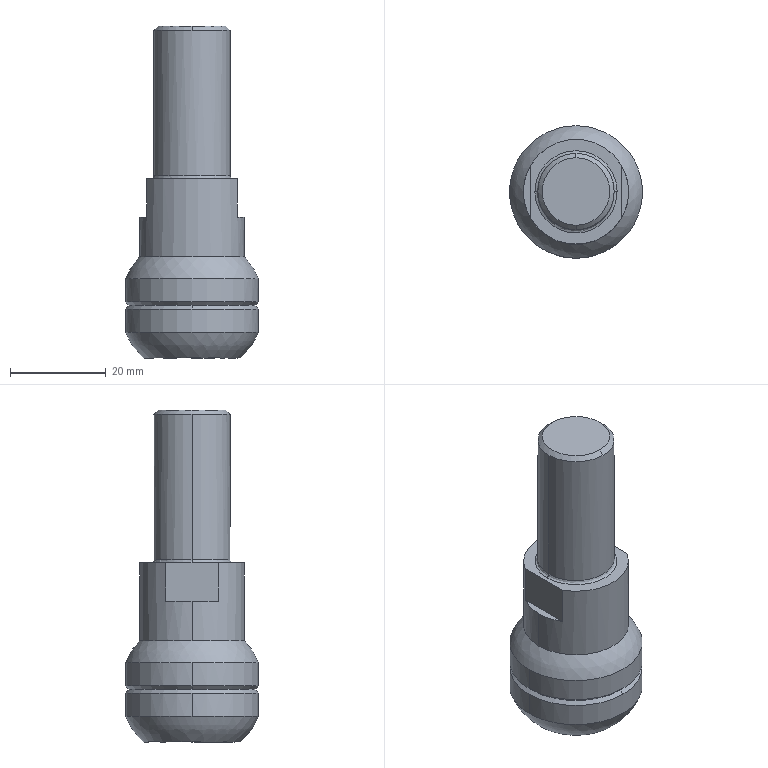Part | SolidWorks | features BaseBody 1 | 1 solid | 25 faces | box 27.8 x 27.8 x 69.5 mm | volume 24116 mm3 | cylinder 8 | plane 7 | cone 6 | spline 4 | commonest cylinder face diameters 27.8 x4 16 x2 22 x2
STEP:
#1=CARTESIAN_POINT('',(8.,0.,0.6));
#2=VERTEX_POINT('',#1);
#3=CARTESIAN_POINT('',(-8.,0.,0.6));
#4=VERTEX_POINT('',#3);
#5=CARTESIAN_POINT('',(0.,0.,0.6));
#6=DIRECTION('',(0.,0.,1.));
#7=DIRECTION('',(1.,0.,0.));
#8=AXIS2_PLACEMENT_3D('',#5,#6,#7);
#9=CIRCLE('',#8,8.);
#10=EDGE_CURVE('',#2,#4,#9,.T.);
#11=ORIENTED_EDGE('',*,*,#10,.F.);
#12=CARTESIAN_POINT('',(8.6,0.,0.));
#13=VERTEX_POINT('',#12);
#14=CARTESIAN_POINT('',(8.6,0.,0.6));
#15=DIRECTION('',(0.,-1.,0.));
#16=DIRECTION('',(1.,0.,0.));
#17=AXIS2_PLACEMENT_3D('',#14,#15,#16);
#18=CIRCLE('',#17,0.6);
#19=EDGE_CURVE('',#2,#13,#18,.T.);
#20=ORIENTED_EDGE('',*,*,#19,.T.);
#21=CARTESIAN_POINT('',(-8.6,0.,0.));
#22=VERTEX_POINT('',#21);
#23=CARTESIAN_POINT('',(-8.6,0.,0.));
#24=CARTESIAN_POINT('',(-8.6,0.2629,0.));
#25=CARTESIAN_POINT('',(-8.582,0.6557,0.));
#26=CARTESIAN_POINT('',(-8.53,1.111,0.));
#27=CARTESIAN_POINT('',(-8.496,1.338,0.));
#28=CARTESIAN_POINT('',(-8.479,1.435,0.));
#29=CARTESIAN_POINT('',(-8.468,1.5,0.));
#30=CARTESIAN_POINT('',(-8.463,1.531,0.));
#31=CARTESIAN_POINT('',(-8.406,1.839,0.));
#32=CARTESIAN_POINT('',(-8.31,2.245,0.));
#33=CARTESIAN_POINT('',(-8.164,2.709,0.));
#34=CARTESIAN_POINT('',(-8.083,2.938,0.));
#35=CARTESIAN_POINT('',(-8.046,3.036,0.));
#36=CARTESIAN_POINT('',(-8.022,3.101,0.));
#37=CARTESIAN_POINT('',(-8.01,3.132,0.));
#38=CARTESIAN_POINT('',(-7.889,3.436,0.));
#39=CARTESIAN_POINT('',(-7.709,3.831,0.));
#40=CARTESIAN_POINT('',(-7.465,4.275,0.));
#41=CARTESIAN_POINT('',(-7.353,4.461,0.));
#42=CARTESIAN_POINT('',(-7.277,4.584,0.));
#43=CARTESIAN_POINT('',(-7.239,4.644,0.));
#44=CARTESIAN_POINT('',(-6.873,5.203,0.));
#45=CARTESIAN_POINT('',(-6.501,5.661,0.));
#46=CARTESIAN_POINT('',(-5.871,6.291,0.));
#47=CARTESIAN_POINT('',(-5.542,6.588,0.));
#48=CARTESIAN_POINT('',(-5.132,6.904,0.));
#49=CARTESIAN_POINT('',(-4.951,7.032,0.));
#50=CARTESIAN_POINT('',(-4.83,7.116,0.));
#51=CARTESIAN_POINT('',(-4.767,7.158,0.));
#52=CARTESIAN_POINT('',(-4.463,7.357,0.));
#53=CARTESIAN_POINT('',(-4.087,7.576,0.));
#54=CARTESIAN_POINT('',(-3.632,7.798,0.));
#55=CARTESIAN_POINT('',(-3.4,7.9,0.));
#56=CARTESIAN_POINT('',(-3.3,7.942,0.));
#57=CARTESIAN_POINT('',(-3.233,7.969,0.));
#58=CARTESIAN_POINT('',(-3.198,7.983,0.));
#59=CARTESIAN_POINT('',(-2.906,8.099,0.));
#60=CARTESIAN_POINT('',(-2.511,8.233,0.));
#61=CARTESIAN_POINT('',(-2.041,8.356,0.));
#62=CARTESIAN_POINT('',(-1.804,8.409,0.));
#63=CARTESIAN_POINT('',(-1.702,8.43,0.));
#64=CARTESIAN_POINT('',(-1.633,8.444,0.));
#65=CARTESIAN_POINT('',(-1.597,8.45,0.));
#66=CARTESIAN_POINT('',(-1.047,8.552,0.));
#67=CARTESIAN_POINT('',(-0.5264,8.6,0.));
#68=CARTESIAN_POINT('',(0.2632,8.6,0.));
#69=CARTESIAN_POINT('',(0.6562,8.582,0.));
#70=CARTESIAN_POINT('',(1.112,8.53,0.));
#71=CARTESIAN_POINT('',(1.338,8.496,0.));
#72=CARTESIAN_POINT('',(1.436,8.479,0.));
#73=CARTESIAN_POINT('',(1.5,8.468,0.));
#74=CARTESIAN_POINT('',(1.531,8.463,0.));
#75=CARTESIAN_POINT('',(1.839,8.406,0.));
#76=CARTESIAN_POINT('',(2.245,8.31,0.));
#77=CARTESIAN_POINT('',(2.709,8.164,0.));
#78=CARTESIAN_POINT('',(2.938,8.083,0.));
#79=CARTESIAN_POINT('',(3.036,8.046,0.));
#80=CARTESIAN_POINT('',(3.101,8.022,0.));
#81=CARTESIAN_POINT('',(3.132,8.01,0.));
#82=CARTESIAN_POINT('',(3.436,7.889,0.));
#83=CARTESIAN_POINT('',(3.831,7.709,0.));
#84=CARTESIAN_POINT('',(4.275,7.465,0.));
#85=CARTESIAN_POINT('',(4.461,7.353,0.));
#86=CARTESIAN_POINT('',(4.584,7.277,0.));
#87=CARTESIAN_POINT('',(4.644,7.239,0.));
#88=CARTESIAN_POINT('',(5.203,6.873,0.));
#89=CARTESIAN_POINT('',(5.661,6.501,0.));
#90=CARTESIAN_POINT('',(6.291,5.871,0.));
#91=CARTESIAN_POINT('',(6.588,5.542,0.));
#92=CARTESIAN_POINT('',(6.904,5.132,0.));
#93=CARTESIAN_POINT('',(7.032,4.951,0.));
#94=CARTESIAN_POINT('',(7.116,4.83,0.));
#95=CARTESIAN_POINT('',(7.158,4.767,0.));
#96=CARTESIAN_POINT('',(7.357,4.463,0.));
#97=CARTESIAN_POINT('',(7.576,4.087,0.));
#98=CARTESIAN_POINT('',(7.798,3.632,0.));
#99=CARTESIAN_POINT('',(7.9,3.4,0.));
#100=CARTESIAN_POINT('',(7.942,3.3,0.));
#101=CARTESIAN_POINT('',(7.969,3.233,0.));
#102=CARTESIAN_POINT('',(7.983,3.198,0.));
#103=CARTESIAN_POINT('',(8.099,2.906,0.));
#104=CARTESIAN_POINT('',(8.233,2.511,0.));
#105=CARTESIAN_POINT('',(8.356,2.041,0.));
#106=CARTESIAN_POINT('',(8.409,1.804,0.));
#107=CARTESIAN_POINT('',(8.43,1.702,0.));
#108=CARTESIAN_POINT('',(8.444,1.633,0.));
#109=CARTESIAN_POINT('',(8.45,1.597,0.));
#110=CARTESIAN_POINT('',(8.552,1.047,0.));
#111=CARTESIAN_POINT('',(8.6,0.5264,0.));
#112=CARTESIAN_POINT('',(8.6,0.,0.));
#113=B_SPLINE_CURVE_WITH_KNOTS('',3,(#23,#24,#25,#26,#27,#28,#29,#30,#31,#32,#33,#34,#35,#36,#37,#38,#39,#40,#41,#42,#43,#44,#45,#46,#47,#48,#49,#50,#51,#52,#53,#54,#55,#56,#57,#58,#59,#60,#61,#62,#63,#64,#65,#66,#67,#68,#69,#70,#71,#72,#73,#74,#75,#76,#77,#78,#79,#80,#81,#82,#83,#84,#85,#86,#87,#88,#89,#90,#91,#92,#93,#94,#95,#96,#97,#98,#99,#100,#101,#102,#103,#104,#105,#106,#107,#108,#109,#110,#111,#112),.UNSPECIFIED.,.F.,.F.,(4,1,1,1,2,2,1,1,1,2,2,1,1,2,2,2,1,1,2,2,1,1,1,2,2,1,1,1,2,2,2,1,1,1,2,2,1,1,1,2,2,1,1,2,2,2,1,1,2,2,1,1,1,2,2,1,1,1,2,2,4),(0.,0.01563,0.02344,0.02734,0.0293,0.03125,0.04688,0.05469,0.05859,0.06055,0.0625,0.07813,0.08594,0.08984,0.09375,0.125,0.1406,0.1484,0.1523,0.1563,0.1719,0.1797,0.1836,0.1855,0.1875,0.2031,0.2109,0.2148,0.2168,0.2188,0.25,0.2656,0.2734,0.2773,0.2793,0.2813,0.2969,0.3047,0.3086,0.3105,0.3125,0.3281,0.3359,0.3398,0.3438,0.375,0.3906,0.3984,0.4023,0.4063,0.4219,0.4297,0.4336,0.4355,0.4375,0.4531,0.4609,0.4648,0.4668,0.4688,0.5),.UNSPECIFIED.);
#114=EDGE_CURVE('',#22,#13,#113,.T.);
#115=ORIENTED_EDGE('',*,*,#114,.F.);
#116=CARTESIAN_POINT('',(-8.6,0.,0.6));
#117=DIRECTION('',(0.,1.,0.));
#118=DIRECTION('',(-1.,0.,0.));
#119=AXIS2_PLACEMENT_3D('',#116,#117,#118);
#120=CIRCLE('',#119,0.6);
#121=EDGE_CURVE('',#4,#22,#120,.T.);
#122=ORIENTED_EDGE('',*,*,#121,.F.);
#123=EDGE_LOOP('',(#11,#20,#115,#122));
#124=FACE_OUTER_BOUND('',#123,.T.);
#125=CARTESIAN_POINT('',(-8.,0.,0.6));
#126=CARTESIAN_POINT('',(-8.,16.,0.6));
#127=CARTESIAN_POINT('',(8.,16.,0.6));
#128=CARTESIAN_POINT('',(8.,0.,0.6));
#129=CARTESIAN_POINT('',(-8.,0.,0.2485));
#130=CARTESIAN_POINT('',(-8.,16.,0.2485));
#131=CARTESIAN_POINT('',(8.,16.,0.2485));
#132=CARTESIAN_POINT('',(8.,0.,0.2485));
#133=CARTESIAN_POINT('',(-8.249,0.,0.));
#134=CARTESIAN_POINT('',(-8.249,16.497,0.));
#135=CARTESIAN_POINT('',(8.249,16.497,0.));
#136=CARTESIAN_POINT('',(8.249,0.,0.));
#137=CARTESIAN_POINT('',(-8.6,0.,0.));
#138=CARTESIAN_POINT('',(-8.6,17.2,0.));
#139=CARTESIAN_POINT('',(8.6,17.2,0.));
#140=CARTESIAN_POINT('',(8.6,0.,0.));
#141=(BOUNDED_SURFACE()B_SPLINE_SURFACE(3,3,((#125,#126,#127,#128),(#129,#130,#131,#132),(#133,#134,#135,#136),(#137,#138,#139,#140)),.UNSPECIFIED.,.F.,.F.,.F.)B_SPLINE_SURFACE_WITH_KNOTS((4,4),(4,4),(0.,1.),(0.,1.),.UNSPECIFIED.)GEOMETRIC_REPRESENTATION_ITEM()RATIONAL_B_SPLINE_SURFACE(((1.,0.3333,0.3333,1.),(0.8047,0.2682,0.2682,0.8047),(0.8047,0.2682,0.2682,0.8047),(1.,0.3333,0.3333,1.)))REPRESENTATION_ITEM('')SURFACE());
#142=ADVANCED_FACE('',(#124),#141,.F.);
#143=ORIENTED_EDGE('',*,*,#10,.T.);
#144=CARTESIAN_POINT('',(-8.,0.,31.08));
#145=VERTEX_POINT('',#144);
#146=CARTESIAN_POINT('',(-8.,0.,-37.5));
#147=DIRECTION('',(0.,0.,1.));
#148=VECTOR('',#147,1000.);
#149=LINE('',#146,#148);
#150=EDGE_CURVE('',#4,#145,#149,.T.);
#151=ORIENTED_EDGE('',*,*,#150,.T.);
#152=CARTESIAN_POINT('',(0.,8.,31.08));
#153=VERTEX_POINT('',#152);
#154=CARTESIAN_POINT('',(0.,0.,31.08));
#155=DIRECTION('',(0.,0.,-1.));
#156=DIRECTION('',(1.,0.,0.));
#157=AXIS2_PLACEMENT_3D('',#154,#155,#156);
#158=CIRCLE('',#157,8.);
#159=EDGE_CURVE('',#145,#153,#158,.T.);
#160=ORIENTED_EDGE('',*,*,#159,.T.);
#161=CARTESIAN_POINT('',(8.,0.,31.08));
#162=VERTEX_POINT('',#161);
#163=CARTESIAN_POINT('',(0.,0.,31.08));
#164=DIRECTION('',(0.,0.,-1.));
#165=DIRECTION('',(1.,0.,0.));
#166=AXIS2_PLACEMENT_3D('',#163,#164,#165);
#167=CIRCLE('',#166,8.);
#168=EDGE_CURVE('',#153,#162,#167,.T.);
#169=ORIENTED_EDGE('',*,*,#168,.T.);
#170=CARTESIAN_POINT('',(8.,0.,-37.5));
#171=DIRECTION('',(0.,0.,1.));
#172=VECTOR('',#171,1000.);
#173=LINE('',#170,#172);
#174=EDGE_CURVE('',#2,#162,#173,.T.);
#175=ORIENTED_EDGE('',*,*,#174,.F.);
#176=EDGE_LOOP('',(#143,#151,#160,#169,#175));
#177=FACE_OUTER_BOUND('',#176,.T.);
#178=CARTESIAN_POINT('',(0.,0.,-37.5));
#179=DIRECTION('',(0.,0.,1.));
#180=DIRECTION('',(1.,0.,0.));
#181=AXIS2_PLACEMENT_3D('',#178,#179,#180);
#182=CYLINDRICAL_SURFACE('',#181,8.);
#183=ADVANCED_FACE('',(#177),#182,.T.);
#184=CARTESIAN_POINT('',(0.,7.08,32.));
#185=VERTEX_POINT('',#184);
#186=CARTESIAN_POINT('',(0.,-7.08,32.));
#187=VERTEX_POINT('',#186);
#188=CARTESIAN_POINT('',(0.,0.,32.));
#189=DIRECTION('',(0.,0.,-1.));
#190=DIRECTION('',(0.,1.,0.));
#191=AXIS2_PLACEMENT_3D('',#188,#189,#190);
#192=CIRCLE('',#191,7.08);
#193=EDGE_CURVE('',#185,#187,#192,.T.);
#194=ORIENTED_EDGE('',*,*,#193,.T.);
#195=CARTESIAN_POINT('',(0.,-8.,31.08));
#196=VERTEX_POINT('',#195);
#197=CARTESIAN_POINT('',(0.,-8.,31.08));
#198=DIRECTION('',(0.,-0.7071,-0.7071));
#199=VECTOR('',#198,1000.);
#200=LINE('',#197,#199);
#201=EDGE_CURVE('',#187,#196,#200,.T.);
#202=ORIENTED_EDGE('',*,*,#201,.T.);
#203=CARTESIAN_POINT('',(0.,0.,31.08));
#204=DIRECTION('',(0.,0.,-1.));
#205=DIRECTION('',(1.,0.,0.));
#206=AXIS2_PLACEMENT_3D('',#203,#204,#205);
#207=CIRCLE('',#206,8.);
#208=EDGE_CURVE('',#162,#196,#207,.T.);
#209=ORIENTED_EDGE('',*,*,#208,.F.);
#210=ORIENTED_EDGE('',*,*,#168,.F.);
#211=CARTESIAN_POINT('',(0.,8.,31.08));
#212=DIRECTION('',(0.,0.7071,-0.7071));
#213=VECTOR('',#212,1000.);
#214=LINE('',#211,#213);
#215=EDGE_CURVE('',#185,#153,#214,.T.);
#216=ORIENTED_EDGE('',*,*,#215,.F.);
#217=EDGE_LOOP('',(#194,#202,#209,#210,#216));
#218=FACE_OUTER_BOUND('',#217,.T.);
#219=CARTESIAN_POINT('',(0.,0.,31.08));
#220=DIRECTION('',(0.,0.,-1.));
#221=DIRECTION('',(0.,1.,0.));
#222=AXIS2_PLACEMENT_3D('',#219,#220,#221);
#223=CONICAL_SURFACE('',#222,8.,0.7854);
#224=ADVANCED_FACE('',(#218),#223,.T.);
#225=CARTESIAN_POINT('',(11.,0.,-16.302));
#226=VERTEX_POINT('',#225);
#227=CARTESIAN_POINT('',(-11.,0.,-16.302));
#228=VERTEX_POINT('',#227);
#229=CARTESIAN_POINT('',(0.,0.,-16.302));
#230=DIRECTION('',(0.,0.,1.));
#231=DIRECTION('',(1.,0.,0.));
#232=AXIS2_PLACEMENT_3D('',#229,#230,#231);
#233=CIRCLE('',#232,11.);
#234=EDGE_CURVE('',#226,#228,#233,.T.);
#235=ORIENTED_EDGE('',*,*,#234,.T.);
#236=CARTESIAN_POINT('',(-11.,0.,-8.));
#237=VERTEX_POINT('',#236);
#238=CARTESIAN_POINT('',(-11.,0.,-37.5));
#239=DIRECTION('',(0.,0.,1.));
#240=VECTOR('',#239,1000.);
#241=LINE('',#238,#240);
#242=EDGE_CURVE('',#228,#237,#241,.T.);
#243=ORIENTED_EDGE('',*,*,#242,.T.);
#244=CARTESIAN_POINT('',(-9.5,5.545,-8.));
#245=VERTEX_POINT('',#244);
#246=CARTESIAN_POINT('',(0.,0.,-8.));
#247=DIRECTION('',(0.,0.,-1.));
#248=DIRECTION('',(1.,0.,0.));
#249=AXIS2_PLACEMENT_3D('',#246,#247,#248);
#250=CIRCLE('',#249,11.);
#251=EDGE_CURVE('',#237,#245,#250,.T.);
#252=ORIENTED_EDGE('',*,*,#251,.T.);
#253=CARTESIAN_POINT('',(-9.5,5.545,0.));
#254=VERTEX_POINT('',#253);
#255=CARTESIAN_POINT('',(-9.5,5.545,8.));
#256=DIRECTION('',(0.,0.,-1.));
#257=VECTOR('',#256,1000.);
#258=LINE('',#255,#257);
#259=EDGE_CURVE('',#254,#245,#258,.T.);
#260=ORIENTED_EDGE('',*,*,#259,.F.);
#261=CARTESIAN_POINT('',(9.5,5.545,0.));
#262=VERTEX_POINT('',#261);
#263=CARTESIAN_POINT('',(0.,0.,0.));
#264=DIRECTION('',(0.,0.,-1.));
#265=DIRECTION('',(1.,0.,0.));
#266=AXIS2_PLACEMENT_3D('',#263,#264,#265);
#267=CIRCLE('',#266,11.);
#268=EDGE_CURVE('',#254,#262,#267,.T.);
#269=ORIENTED_EDGE('',*,*,#268,.T.);
#270=CARTESIAN_POINT('',(9.5,5.545,-8.));
#271=VERTEX_POINT('',#270);
#272=CARTESIAN_POINT('',(9.5,5.545,-37.5));
#273=DIRECTION('',(0.,0.,-1.));
#274=VECTOR('',#273,1000.);
#275=LINE('',#272,#274);
#276=EDGE_CURVE('',#262,#271,#275,.T.);
#277=ORIENTED_EDGE('',*,*,#276,.T.);
#278=CARTESIAN_POINT('',(11.,0.,-8.));
#279=VERTEX_POINT('',#278);
#280=CARTESIAN_POINT('',(0.,0.,-8.));
#281=DIRECTION('',(0.,0.,-1.));
#282=DIRECTION('',(1.,0.,0.));
#283=AXIS2_PLACEMENT_3D('',#280,#281,#282);
#284=CIRCLE('',#283,11.);
#285=EDGE_CURVE('',#271,#279,#284,.T.);
#286=ORIENTED_EDGE('',*,*,#285,.T.);
#287=CARTESIAN_POINT('',(11.,0.,-37.5));
#288=DIRECTION('',(0.,0.,1.));
#289=VECTOR('',#288,1000.);
#290=LINE('',#287,#289);
#291=EDGE_CURVE('',#226,#279,#290,.T.);
#292=ORIENTED_EDGE('',*,*,#291,.F.);
#293=EDGE_LOOP('',(#235,#243,#252,#260,#269,#277,#286,#292));
#294=FACE_OUTER_BOUND('',#293,.T.);
#295=CARTESIAN_POINT('',(0.,0.,-37.5));
#296=DIRECTION('',(0.,0.,1.));
#297=DIRECTION('',(1.,0.,0.));
#298=AXIS2_PLACEMENT_3D('',#295,#296,#297);
#299=CYLINDRICAL_SURFACE('',#298,11.);
#300=ADVANCED_FACE('',(#294),#299,.T.);
#301=CARTESIAN_POINT('',(13.9,0.,-25.75));
#302=VERTEX_POINT('',#301);
#303=CARTESIAN_POINT('',(-13.9,0.,-25.75));
#304=VERTEX_POINT('',#303);
#305=CARTESIAN_POINT('',(0.,0.,-25.75));
#306=DIRECTION('',(0.,0.,1.));
#307=DIRECTION('',(1.,0.,0.));
#308=AXIS2_PLACEMENT_3D('',#305,#306,#307);
#309=CIRCLE('',#308,13.9);
#310=EDGE_CURVE('',#302,#304,#309,.T.);
#311=ORIENTED_EDGE('',*,*,#310,.T.);
#312=CARTESIAN_POINT('',(-13.9,0.,-20.862));
#313=VERTEX_POINT('',#312);
#314=CARTESIAN_POINT('',(-13.9,0.,-37.5));
#315=DIRECTION('',(0.,0.,1.));
#316=VECTOR('',#315,1000.);
#317=LINE('',#314,#316);
#318=EDGE_CURVE('',#304,#313,#317,.T.);
#319=ORIENTED_EDGE('',*,*,#318,.T.);
#320=CARTESIAN_POINT('',(13.9,0.,-20.862));
#321=VERTEX_POINT('',#320);
#322=CARTESIAN_POINT('',(0.,0.,-20.862));
#323=DIRECTION('',(0.,0.,1.));
#324=DIRECTION('',(1.,0.,0.));
#325=AXIS2_PLACEMENT_3D('',#322,#323,#324);
#326=CIRCLE('',#325,13.9);
#327=EDGE_CURVE('',#321,#313,#326,.T.);
#328=ORIENTED_EDGE('',*,*,#327,.F.);
#329=CARTESIAN_POINT('',(13.9,0.,-37.5));
#330=DIRECTION('',(0.,0.,1.));
#331=VECTOR('',#330,1000.);
#332=LINE('',#329,#331);
#333=EDGE_CURVE('',#302,#321,#332,.T.);
#334=ORIENTED_EDGE('',*,*,#333,.F.);
#335=EDGE_LOOP('',(#311,#319,#328,#334));
#336=FACE_OUTER_BOUND('',#335,.T.);
#337=CARTESIAN_POINT('',(0.,0.,-37.5));
#338=DIRECTION('',(0.,0.,1.));
#339=DIRECTION('',(1.,0.,0.));
#340=AXIS2_PLACEMENT_3D('',#337,#338,#339);
#341=CYLINDRICAL_SURFACE('',#340,13.9);
#342=ADVANCED_FACE('',(#336),#341,.T.);
#343=CARTESIAN_POINT('',(0.,13.15,-26.5));
#344=VERTEX_POINT('',#343);
#345=CARTESIAN_POINT('',(-13.15,0.,-26.5));
#346=VERTEX_POINT('',#345);
#347=CARTESIAN_POINT('',(0.,0.,-26.5));
#348=DIRECTION('',(0.,0.,1.));
#349=DIRECTION('',(1.,0.,0.));
#350=AXIS2_PLACEMENT_3D('',#347,#348,#349);
#351=CIRCLE('',#350,13.15);
#352=EDGE_CURVE('',#344,#346,#351,.T.);
#353=ORIENTED_EDGE('',*,*,#352,.T.);
#354=CARTESIAN_POINT('',(-13.9,0.,-25.75));
#355=DIRECTION('',(-0.7071,0.,0.7071));
#356=VECTOR('',#355,1000.);
#357=LINE('',#354,#356);
#358=EDGE_CURVE('',#346,#304,#357,.T.);
#359=ORIENTED_EDGE('',*,*,#358,.T.);
#360=ORIENTED_EDGE('',*,*,#310,.F.);
#361=CARTESIAN_POINT('',(13.15,0.,-26.5));
#362=VERTEX_POINT('',#361);
#363=CARTESIAN_POINT('',(13.9,0.,-25.75));
#364=DIRECTION('',(0.7071,0.,0.7071));
#365=VECTOR('',#364,1000.);
#366=LINE('',#363,#365);
#367=EDGE_CURVE('',#362,#302,#366,.T.);
#368=ORIENTED_EDGE('',*,*,#367,.F.);
#369=CARTESIAN_POINT('',(0.,0.,-26.5));
#370=DIRECTION('',(0.,0.,1.));
#371=DIRECTION('',(1.,0.,0.));
#372=AXIS2_PLACEMENT_3D('',#369,#370,#371);
#373=CIRCLE('',#372,13.15);
#374=EDGE_CURVE('',#362,#344,#373,.T.);
#375=ORIENTED_EDGE('',*,*,#374,.T.);
#376=EDGE_LOOP('',(#353,#359,#360,#368,#375));
#377=FACE_OUTER_BOUND('',#376,.T.);
#378=CARTESIAN_POINT('',(0.,0.,-25.75));
#379=DIRECTION('',(0.,0.,1.));
#380=DIRECTION('',(1.,0.,0.));
#381=AXIS2_PLACEMENT_3D('',#378,#379,#380);
#382=CONICAL_SURFACE('',#381,13.9,0.7854);
#383=ADVANCED_FACE('',(#377),#382,.T.);
#384=CARTESIAN_POINT('',(0.,-13.15,-26.5));
#385=VERTEX_POINT('',#384);
#386=CARTESIAN_POINT('',(0.,0.,-26.5));
#387=DIRECTION('',(0.,0.,1.));
#388=DIRECTION('',(1.,0.,0.));
#389=AXIS2_PLACEMENT_3D('',#386,#387,#388);
#390=CIRCLE('',#389,13.15);
#391=EDGE_CURVE('',#385,#362,#390,.T.);
#392=ORIENTED_EDGE('',*,*,#391,.F.);
#393=CARTESIAN_POINT('',(0.,-13.9,-27.25));
#394=VERTEX_POINT('',#393);
#395=CARTESIAN_POINT('',(0.,-13.9,-27.25));
#396=DIRECTION('',(0.,-0.7071,-0.7071));
#397=VECTOR('',#396,1000.);
#398=LINE('',#395,#397);
#399=EDGE_CURVE('',#385,#394,#398,.T.);
#400=ORIENTED_EDGE('',*,*,#399,.T.);
#401=CARTESIAN_POINT('',(13.9,0.,-27.25));
#402=VERTEX_POINT('',#401);
#403=CARTESIAN_POINT('',(0.,0.,-27.25));
#404=DIRECTION('',(0.,0.,1.));
#405=DIRECTION('',(-1.,0.,0.));
#406=AXIS2_PLACEMENT_3D('',#403,#404,#405);
#407=CIRCLE('',#406,13.9);
#408=EDGE_CURVE('',#394,#402,#407,.T.);
#409=ORIENTED_EDGE('',*,*,#408,.T.);
#410=CARTESIAN_POINT('',(0.,13.9,-27.25));
#411=VERTEX_POINT('',#410);
#412=CARTESIAN_POINT('',(0.,0.,-27.25));
#413=DIRECTION('',(0.,0.,1.));
#414=DIRECTION('',(-1.,0.,0.));
#415=AXIS2_PLACEMENT_3D('',#412,#413,#414);
#416=CIRCLE('',#415,13.9);
#417=EDGE_CURVE('',#402,#411,#416,.T.);
#418=ORIENTED_EDGE('',*,*,#417,.T.);
#419=CARTESIAN_POINT('',(0.,13.9,-27.25));
#420=DIRECTION('',(0.,0.7071,-0.7071));
#421=VECTOR('',#420,1000.);
#422=LINE('',#419,#421);
#423=EDGE_CURVE('',#344,#411,#422,.T.);
#424=ORIENTED_EDGE('',*,*,#423,.F.);
#425=ORIENTED_EDGE('',*,*,#374,.F.);
#426=EDGE_LOOP('',(#392,#400,#409,#418,#424,#425));
#427=FACE_OUTER_BOUND('',#426,.T.);
#428=CARTESIAN_POINT('',(0.,0.,-27.25));
#429=DIRECTION('',(0.,0.,-1.));
#430=DIRECTION('',(0.,1.,0.));
#431=AXIS2_PLACEMENT_3D('',#428,#429,#430);
#432=CONICAL_SURFACE('',#431,13.9,0.7854);
#433=ADVANCED_FACE('',(#427),#432,.T.);
#434=CARTESIAN_POINT('',(13.9,0.,-32.138));
#435=VERTEX_POINT('',#434);
#436=CARTESIAN_POINT('',(-13.9,0.,-32.138));
#437=VERTEX_POINT('',#436);
#438=CARTESIAN_POINT('',(0.,0.,-32.138));
#439=DIRECTION('',(0.,0.,1.));
#440=DIRECTION('',(1.,0.,0.));
#441=AXIS2_PLACEMENT_3D('',#438,#439,#440);
#442=CIRCLE('',#441,13.9);
#443=EDGE_CURVE('',#435,#437,#442,.T.);
#444=ORIENTED_EDGE('',*,*,#443,.T.);
#445=CARTESIAN_POINT('',(-13.9,0.,-27.25));
#446=VERTEX_POINT('',#445);
#447=CARTESIAN_POINT('',(-13.9,0.,-37.5));
#448=DIRECTION('',(0.,0.,1.));
#449=VECTOR('',#448,1000.);
#450=LINE('',#447,#449);
#451=EDGE_CURVE('',#437,#446,#450,.T.);
#452=ORIENTED_EDGE('',*,*,#451,.T.);
#453=CARTESIAN_POINT('',(0.,0.,-27.25));
#454=DIRECTION('',(0.,0.,1.));
#455=DIRECTION('',(-1.,0.,0.));
#456=AXIS2_PLACEMENT_3D('',#453,#454,#455);
#457=CIRCLE('',#456,13.9);
#458=EDGE_CURVE('',#411,#446,#457,.T.);
#459=ORIENTED_EDGE('',*,*,#458,.F.);
#460=ORIENTED_EDGE('',*,*,#417,.F.);
#461=CARTESIAN_POINT('',(13.9,0.,-37.5));
#462=DIRECTION('',(0.,0.,1.));
#463=VECTOR('',#462,1000.);
#464=LINE('',#461,#463);
#465=EDGE_CURVE('',#435,#402,#464,.T.);
#466=ORIENTED_EDGE('',*,*,#465,.F.);
#467=EDGE_LOOP('',(#444,#452,#459,#460,#466));
#468=FACE_OUTER_BOUND('',#467,.T.);
#469=CARTESIAN_POINT('',(0.,0.,-37.5));
#470=DIRECTION('',(0.,0.,1.));
#471=DIRECTION('',(1.,0.,0.));
#472=AXIS2_PLACEMENT_3D('',#469,#470,#471);
#473=CYLINDRICAL_SURFACE('',#472,13.9);
#474=ADVANCED_FACE('',(#468),#473,.T.);
#475=ORIENTED_EDGE('',*,*,#150,.F.);
#476=CARTESIAN_POINT('',(0.,0.,0.6));
#477=DIRECTION('',(0.,0.,1.));
#478=DIRECTION('',(1.,0.,0.));
#479=AXIS2_PLACEMENT_3D('',#476,#477,#478);
#480=CIRCLE('',#479,8.);
#481=EDGE_CURVE('',#4,#2,#480,.T.);
#482=ORIENTED_EDGE('',*,*,#481,.T.);
#483=ORIENTED_EDGE('',*,*,#174,.T.);
#484=ORIENTED_EDGE('',*,*,#208,.T.);
#485=CARTESIAN_POINT('',(0.,0.,31.08));
#486=DIRECTION('',(0.,0.,-1.));
#487=DIRECTION('',(1.,0.,0.));
#488=AXIS2_PLACEMENT_3D('',#485,#486,#487);
#489=CIRCLE('',#488,8.);
#490=EDGE_CURVE('',#196,#145,#489,.T.);
#491=ORIENTED_EDGE('',*,*,#490,.T.);
#492=EDGE_LOOP('',(#475,#482,#483,#484,#491));
#493=FACE_OUTER_BOUND('',#492,.T.);
#494=CARTESIAN_POINT('',(0.,0.,-37.5));
#495=DIRECTION('',(0.,0.,1.));
#496=DIRECTION('',(1.,0.,0.));
#497=AXIS2_PLACEMENT_3D('',#494,#495,#496);
#498=CYLINDRICAL_SURFACE('',#497,8.);
#499=ADVANCED_FACE('',(#493),#498,.T.);
#500=ORIENTED_EDGE('',*,*,#201,.F.);
#501=CARTESIAN_POINT('',(0.,0.,32.));
#502=DIRECTION('',(0.,0.,-1.));
#503=DIRECTION('',(0.,1.,0.));
#504=AXIS2_PLACEMENT_3D('',#501,#502,#503);
#505=CIRCLE('',#504,7.08);
#506=EDGE_CURVE('',#187,#185,#505,.T.);
#507=ORIENTED_EDGE('',*,*,#506,.T.);
#508=ORIENTED_EDGE('',*,*,#215,.T.);
#509=ORIENTED_EDGE('',*,*,#159,.F.);
#510=ORIENTED_EDGE('',*,*,#490,.F.);
#511=EDGE_LOOP('',(#500,#507,#508,#509,#510));
#512=FACE_OUTER_BOUND('',#511,.T.);
#513=CARTESIAN_POINT('',(0.,0.,31.08));
#514=DIRECTION('',(0.,0.,-1.));
#515=DIRECTION('',(0.,1.,0.));
#516=AXIS2_PLACEMENT_3D('',#513,#514,#515);
#517=CONICAL_SURFACE('',#516,8.,0.7854);
#518=ADVANCED_FACE('',(#512),#517,.T.);
#519=ORIENTED_EDGE('',*,*,#19,.F.);
#520=ORIENTED_EDGE('',*,*,#481,.F.);
#521=ORIENTED_EDGE('',*,*,#121,.T.);
#522=CARTESIAN_POINT('',(8.6,0.,0.));
#523=CARTESIAN_POINT('',(8.6,-0.2632,0.));
#524=CARTESIAN_POINT('',(8.582,-0.6562,0.));
#525=CARTESIAN_POINT('',(8.53,-1.112,0.));
#526=CARTESIAN_POINT('',(8.496,-1.338,0.));
#527=CARTESIAN_POINT('',(8.479,-1.436,0.));
#528=CARTESIAN_POINT('',(8.468,-1.5,0.));
#529=CARTESIAN_POINT('',(8.463,-1.531,0.));
#530=CARTESIAN_POINT('',(8.406,-1.839,0.));
#531=CARTESIAN_POINT('',(8.31,-2.245,0.));
#532=CARTESIAN_POINT('',(8.164,-2.709,0.));
#533=CARTESIAN_POINT('',(8.083,-2.938,0.));
#534=CARTESIAN_POINT('',(8.046,-3.036,0.));
#535=CARTESIAN_POINT('',(8.022,-3.101,0.));
#536=CARTESIAN_POINT('',(8.01,-3.132,0.));
#537=CARTESIAN_POINT('',(7.889,-3.436,0.));
#538=CARTESIAN_POINT('',(7.709,-3.831,0.));
#539=CARTESIAN_POINT('',(7.465,-4.275,0.));
#540=CARTESIAN_POINT('',(7.353,-4.461,0.));
#541=CARTESIAN_POINT('',(7.277,-4.584,0.));
#542=CARTESIAN_POINT('',(7.239,-4.644,0.));
#543=CARTESIAN_POINT('',(6.873,-5.203,0.));
#544=CARTESIAN_POINT('',(6.501,-5.661,0.));
#545=CARTESIAN_POINT('',(5.871,-6.291,0.));
#546=CARTESIAN_POINT('',(5.542,-6.588,0.));
#547=CARTESIAN_POINT('',(5.132,-6.904,0.));
#548=CARTESIAN_POINT('',(4.951,-7.032,0.));
#549=CARTESIAN_POINT('',(4.83,-7.116,0.));
#550=CARTESIAN_POINT('',(4.767,-7.158,0.));
#551=CARTESIAN_POINT('',(4.463,-7.357,0.));
#552=CARTESIAN_POINT('',(4.087,-7.576,0.));
#553=CARTESIAN_POINT('',(3.632,-7.798,0.));
#554=CARTESIAN_POINT('',(3.4,-7.9,0.));
#555=CARTESIAN_POINT('',(3.3,-7.942,0.));
#556=CARTESIAN_POINT('',(3.233,-7.969,0.));
#557=CARTESIAN_POINT('',(3.198,-7.983,0.));
#558=CARTESIAN_POINT('',(2.906,-8.099,0.));
#559=CARTESIAN_POINT('',(2.511,-8.233,0.));
#560=CARTESIAN_POINT('',(2.041,-8.356,0.));
#561=CARTESIAN_POINT('',(1.804,-8.409,0.));
#562=CARTESIAN_POINT('',(1.702,-8.43,0.));
#563=CARTESIAN_POINT('',(1.633,-8.444,0.));
#564=CARTESIAN_POINT('',(1.597,-8.45,0.));
#565=CARTESIAN_POINT('',(1.047,-8.552,0.));
#566=CARTESIAN_POINT('',(0.5264,-8.6,0.));
#567=CARTESIAN_POINT('',(-0.2632,-8.6,0.));
#568=CARTESIAN_POINT('',(-0.6562,-8.582,0.));
#569=CARTESIAN_POINT('',(-1.112,-8.53,0.));
#570=CARTESIAN_POINT('',(-1.338,-8.496,0.));
#571=CARTESIAN_POINT('',(-1.436,-8.479,0.));
#572=CARTESIAN_POINT('',(-1.5,-8.468,0.));
#573=CARTESIAN_POINT('',(-1.531,-8.463,0.));
#574=CARTESIAN_POINT('',(-1.839,-8.406,0.));
#575=CARTESIAN_POINT('',(-2.245,-8.31,0.));
#576=CARTESIAN_POINT('',(-2.709,-8.164,0.));
#577=CARTESIAN_POINT('',(-2.938,-8.083,0.));
#578=CARTESIAN_POINT('',(-3.036,-8.046,0.));
#579=CARTESIAN_POINT('',(-3.101,-8.022,0.));
#580=CARTESIAN_POINT('',(-3.132,-8.01,0.));
#581=CARTESIAN_POINT('',(-3.436,-7.889,0.));
#582=CARTESIAN_POINT('',(-3.831,-7.709,0.));
#583=CARTESIAN_POINT('',(-4.275,-7.465,0.));
#584=CARTESIAN_POINT('',(-4.461,-7.353,0.));
#585=CARTESIAN_POINT('',(-4.584,-7.277,0.));
#586=CARTESIAN_POINT('',(-4.644,-7.239,0.));
#587=CARTESIAN_POINT('',(-5.203,-6.873,0.));
#588=CARTESIAN_POINT('',(-5.661,-6.501,0.));
#589=CARTESIAN_POINT('',(-6.291,-5.871,0.));
#590=CARTESIAN_POINT('',(-6.588,-5.542,0.));
#591=CARTESIAN_POINT('',(-6.904,-5.132,0.));
#592=CARTESIAN_POINT('',(-7.032,-4.951,0.));
#593=CARTESIAN_POINT('',(-7.116,-4.83,0.));
#594=CARTESIAN_POINT('',(-7.158,-4.767,0.));
#595=CARTESIAN_POINT('',(-7.357,-4.463,0.));
#596=CARTESIAN_POINT('',(-7.576,-4.087,0.));
#597=CARTESIAN_POINT('',(-7.798,-3.632,0.));
#598=CARTESIAN_POINT('',(-7.9,-3.4,0.));
#599=CARTESIAN_POINT('',(-7.942,-3.3,0.));
#600=CARTESIAN_POINT('',(-7.969,-3.233,0.));
#601=CARTESIAN_POINT('',(-7.983,-3.198,0.));
#602=CARTESIAN_POINT('',(-8.099,-2.906,0.));
#603=CARTESIAN_POINT('',(-8.233,-2.511,0.));
#604=CARTESIAN_POINT('',(-8.356,-2.041,0.));
#605=CARTESIAN_POINT('',(-8.409,-1.804,0.));
#606=CARTESIAN_POINT('',(-8.43,-1.702,0.));
#607=CARTESIAN_POINT('',(-8.444,-1.633,0.));
#608=CARTESIAN_POINT('',(-8.45,-1.597,0.));
#609=CARTESIAN_POINT('',(-8.552,-1.048,0.));
#610=CARTESIAN_POINT('',(-8.6,-0.5262,0.));
#611=CARTESIAN_POINT('',(-8.6,0.,0.));
#612=B_SPLINE_CURVE_WITH_KNOTS('',3,(#522,#523,#524,#525,#526,#527,#528,#529,#530,#531,#532,#533,#534,#535,#536,#537,#538,#539,#540,#541,#542,#543,#544,#545,#546,#547,#548,#549,#550,#551,#552,#553,#554,#555,#556,#557,#558,#559,#560,#561,#562,#563,#564,#565,#566,#567,#568,#569,#570,#571,#572,#573,#574,#575,#576,#577,#578,#579,#580,#581,#582,#583,#584,#585,#586,#587,#588,#589,#590,#591,#592,#593,#594,#595,#596,#597,#598,#599,#600,#601,#602,#603,#604,#605,#606,#607,#608,#609,#610,#611),.UNSPECIFIED.,.F.,.F.,(4,1,1,1,2,2,1,1,1,2,2,1,1,2,2,2,1,1,2,2,1,1,1,2,2,1,1,1,2,2,2,1,1,1,2,2,1,1,1,2,2,1,1,2,2,2,1,1,2,2,1,1,1,2,2,1,1,1,2,2,4),(0.5,0.5156,0.5234,0.5273,0.5293,0.5313,0.5469,0.5547,0.5586,0.5605,0.5625,0.5781,0.5859,0.5898,0.5938,0.625,0.6406,0.6484,0.6523,0.6562,0.6719,0.6797,0.6836,0.6855,0.6875,0.7031,0.7109,0.7148,0.7168,0.7187,0.75,0.7656,0.7734,0.7773,0.7793,0.7812,0.7969,0.8047,0.8086,0.8105,0.8125,0.8281,0.8359,0.8398,0.8437,0.875,0.8906,0.8984,0.9023,0.9062,0.9219,0.9297,0.9336,0.9355,0.9375,0.9531,0.9609,0.9648,0.9668,0.9687,1.),.UNSPECIFIED.);
#613=EDGE_CURVE('',#13,#22,#612,.T.);
#614=ORIENTED_EDGE('',*,*,#613,.F.);
#615=EDGE_LOOP('',(#519,#520,#521,#614));
#616=FACE_OUTER_BOUND('',#615,.T.);
#617=CARTESIAN_POINT('',(8.,0.,0.6));
#618=CARTESIAN_POINT('',(8.,-16.,0.6));
#619=CARTESIAN_POINT('',(-8.,-16.,0.6));
#620=CARTESIAN_POINT('',(-8.,0.,0.6));
#621=CARTESIAN_POINT('',(8.,0.,0.2485));
#622=CARTESIAN_POINT('',(8.,-16.,0.2485));
#623=CARTESIAN_POINT('',(-8.,-16.,0.2485));
#624=CARTESIAN_POINT('',(-8.,0.,0.2485));
#625=CARTESIAN_POINT('',(8.249,0.,0.));
#626=CARTESIAN_POINT('',(8.249,-16.497,0.));
#627=CARTESIAN_POINT('',(-8.249,-16.497,0.));
#628=CARTESIAN_POINT('',(-8.249,0.,0.));
#629=CARTESIAN_POINT('',(8.6,0.,0.));
#630=CARTESIAN_POINT('',(8.6,-17.2,0.));
#631=CARTESIAN_POINT('',(-8.6,-17.2,0.));
#632=CARTESIAN_POINT('',(-8.6,0.,0.));
#633=(BOUNDED_SURFACE()B_SPLINE_SURFACE(3,3,((#617,#618,#619,#620),(#621,#622,#623,#624),(#625,#626,#627,#628),(#629,#630,#631,#632)),.UNSPECIFIED.,.F.,.F.,.F.)B_SPLINE_SURFACE_WITH_KNOTS((4,4),(4,4),(0.,1.),(0.,1.),.UNSPECIFIED.)GEOMETRIC_REPRESENTATION_ITEM()RATIONAL_B_SPLINE_SURFACE(((1.,0.3333,0.3333,1.),(0.8047,0.2682,0.2682,0.8047),(0.8047,0.2682,0.2682,0.8047),(1.,0.3333,0.3333,1.)))REPRESENTATION_ITEM('')SURFACE());
#634=ADVANCED_FACE('',(#616),#633,.F.);
#635=ORIENTED_EDGE('',*,*,#193,.F.);
#636=ORIENTED_EDGE('',*,*,#506,.F.);
#637=EDGE_LOOP('',(#635,#636));
#638=FACE_OUTER_BOUND('',#637,.T.);
#639=CARTESIAN_POINT('',(0.,0.,32.));
#640=DIRECTION('',(0.,0.,-1.));
#641=DIRECTION('',(-1.,0.,0.));
#642=AXIS2_PLACEMENT_3D('',#639,#640,#641);
#643=PLANE('',#642);
#644=ADVANCED_FACE('',(#638),#643,.F.);
#645=ORIENTED_EDGE('',*,*,#114,.T.);
#646=ORIENTED_EDGE('',*,*,#613,.T.);
#647=EDGE_LOOP('',(#645,#646));
#648=FACE_BOUND('',#647,.T.);
#649=CARTESIAN_POINT('',(9.5,-5.545,0.));
#650=VERTEX_POINT('',#649);
#651=CARTESIAN_POINT('',(-9.5,-5.545,0.));
#652=VERTEX_POINT('',#651);
#653=CARTESIAN_POINT('',(0.,0.,0.));
#654=DIRECTION('',(0.,0.,-1.));
#655=DIRECTION('',(1.,0.,0.));
#656=AXIS2_PLACEMENT_3D('',#653,#654,#655);
#657=CIRCLE('',#656,11.);
#658=EDGE_CURVE('',#650,#652,#657,.T.);
#659=ORIENTED_EDGE('',*,*,#658,.F.);
#660=CARTESIAN_POINT('',(9.5,0.,0.));
#661=DIRECTION('',(0.,-1.,0.));
#662=VECTOR('',#661,1000.);
#663=LINE('',#660,#662);
#664=EDGE_CURVE('',#262,#650,#663,.T.);
#665=ORIENTED_EDGE('',*,*,#664,.F.);
#666=ORIENTED_EDGE('',*,*,#268,.F.);
#667=CARTESIAN_POINT('',(-9.5,0.,0.));
#668=DIRECTION('',(0.,1.,0.));
#669=VECTOR('',#668,1000.);
#670=LINE('',#667,#669);
#671=EDGE_CURVE('',#652,#254,#670,.T.);
#672=ORIENTED_EDGE('',*,*,#671,.F.);
#673=EDGE_LOOP('',(#659,#665,#666,#672));
#674=FACE_OUTER_BOUND('',#673,.T.);
#675=CARTESIAN_POINT('',(-8.6,0.,0.));
#676=DIRECTION('',(0.,0.,-1.));
#677=DIRECTION('',(-1.,0.,0.));
#678=AXIS2_PLACEMENT_3D('',#675,#676,#677);
#679=PLANE('',#678);
#680=ADVANCED_FACE('',(#648,#674),#679,.F.);
#681=CARTESIAN_POINT('',(-9.5,-5.545,-8.));
#682=VERTEX_POINT('',#681);
#683=CARTESIAN_POINT('',(-9.5,-5.545,8.));
#684=DIRECTION('',(0.,0.,1.));
#685=VECTOR('',#684,1000.);
#686=LINE('',#683,#685);
#687=EDGE_CURVE('',#682,#652,#686,.T.);
#688=ORIENTED_EDGE('',*,*,#687,.T.);
#689=ORIENTED_EDGE('',*,*,#671,.T.);
#690=ORIENTED_EDGE('',*,*,#259,.T.);
#691=CARTESIAN_POINT('',(-9.5,-15.,-8.));
#692=DIRECTION('',(0.,-1.,0.));
#693=VECTOR('',#692,1000.);
#694=LINE('',#691,#693);
#695=EDGE_CURVE('',#245,#682,#694,.T.);
#696=ORIENTED_EDGE('',*,*,#695,.T.);
#697=EDGE_LOOP('',(#688,#689,#690,#696));
#698=FACE_OUTER_BOUND('',#697,.T.);
#699=CARTESIAN_POINT('',(-9.5,-15.,8.));
#700=DIRECTION('',(-1.,0.,0.));
#701=DIRECTION('',(0.,0.,1.));
#702=AXIS2_PLACEMENT_3D('',#699,#700,#701);
#703=PLANE('',#702);
#704=ADVANCED_FACE('',(#698),#703,.T.);
#705=ORIENTED_EDGE('',*,*,#242,.F.);
#706=CARTESIAN_POINT('',(0.,0.,-16.302));
#707=DIRECTION('',(0.,0.,1.));
#708=DIRECTION('',(1.,0.,0.));
#709=AXIS2_PLACEMENT_3D('',#706,#707,#708);
#710=CIRCLE('',#709,11.);
#711=EDGE_CURVE('',#228,#226,#710,.T.);
#712=ORIENTED_EDGE('',*,*,#711,.T.);
#713=ORIENTED_EDGE('',*,*,#291,.T.);
#714=CARTESIAN_POINT('',(9.5,-5.545,-8.));
#715=VERTEX_POINT('',#714);
#716=CARTESIAN_POINT('',(0.,0.,-8.));
#717=DIRECTION('',(0.,0.,-1.));
#718=DIRECTION('',(1.,0.,0.));
#719=AXIS2_PLACEMENT_3D('',#716,#717,#718);
#720=CIRCLE('',#719,11.);
#721=EDGE_CURVE('',#279,#715,#720,.T.);
#722=ORIENTED_EDGE('',*,*,#721,.T.);
#723=CARTESIAN_POINT('',(9.5,-5.545,-37.5));
#724=DIRECTION('',(0.,0.,1.));
#725=VECTOR('',#724,1000.);
#726=LINE('',#723,#725);
#727=EDGE_CURVE('',#715,#650,#726,.T.);
#728=ORIENTED_EDGE('',*,*,#727,.T.);
#729=ORIENTED_EDGE('',*,*,#658,.T.);
#730=ORIENTED_EDGE('',*,*,#687,.F.);
#731=CARTESIAN_POINT('',(0.,0.,-8.));
#732=DIRECTION('',(0.,0.,-1.));
#733=DIRECTION('',(1.,0.,0.));
#734=AXIS2_PLACEMENT_3D('',#731,#732,#733);
#735=CIRCLE('',#734,11.);
#736=EDGE_CURVE('',#682,#237,#735,.T.);
#737=ORIENTED_EDGE('',*,*,#736,.T.);
#738=EDGE_LOOP('',(#705,#712,#713,#722,#728,#729,#730,#737));
#739=FACE_OUTER_BOUND('',#738,.T.);
#740=CARTESIAN_POINT('',(0.,0.,-37.5));
#741=DIRECTION('',(0.,0.,1.));
#742=DIRECTION('',(1.,0.,0.));
#743=AXIS2_PLACEMENT_3D('',#740,#741,#742);
#744=CYLINDRICAL_SURFACE('',#743,11.);
#745=ADVANCED_FACE('',(#739),#744,.T.);
#746=ORIENTED_EDGE('',*,*,#276,.F.);
#747=ORIENTED_EDGE('',*,*,#664,.T.);
#748=ORIENTED_EDGE('',*,*,#727,.F.);
#749=CARTESIAN_POINT('',(9.5,10.,-8.));
#750=DIRECTION('',(0.,1.,0.));
#751=VECTOR('',#750,1000.);
#752=LINE('',#749,#751);
#753=EDGE_CURVE('',#715,#271,#752,.T.);
#754=ORIENTED_EDGE('',*,*,#753,.T.);
#755=EDGE_LOOP('',(#746,#747,#748,#754));
#756=FACE_OUTER_BOUND('',#755,.T.);
#757=CARTESIAN_POINT('',(9.5,10.,8.));
#758=DIRECTION('',(1.,0.,0.));
#759=DIRECTION('',(0.,0.,-1.));
#760=AXIS2_PLACEMENT_3D('',#757,#758,#759);
#761=PLANE('',#760);
#762=ADVANCED_FACE('',(#756),#761,.T.);
#763=ORIENTED_EDGE('',*,*,#695,.F.);
#764=ORIENTED_EDGE('',*,*,#251,.F.);
#765=ORIENTED_EDGE('',*,*,#736,.F.);
#766=EDGE_LOOP('',(#763,#764,#765));
#767=FACE_OUTER_BOUND('',#766,.T.);
#768=CARTESIAN_POINT('',(0.,0.,-8.));
#769=DIRECTION('',(0.,0.,1.));
#770=DIRECTION('',(1.,0.,0.));
#771=AXIS2_PLACEMENT_3D('',#768,#769,#770);
#772=PLANE('',#771);
#773=ADVANCED_FACE('',(#767),#772,.T.);
#774=ORIENTED_EDGE('',*,*,#285,.F.);
#775=ORIENTED_EDGE('',*,*,#753,.F.);
#776=ORIENTED_EDGE('',*,*,#721,.F.);
#777=EDGE_LOOP('',(#774,#775,#776));
#778=FACE_OUTER_BOUND('',#777,.T.);
#779=CARTESIAN_POINT('',(0.,0.,-8.));
#780=DIRECTION('',(0.,0.,1.));
#781=DIRECTION('',(1.,0.,0.));
#782=AXIS2_PLACEMENT_3D('',#779,#780,#781);
#783=PLANE('',#782);
#784=ADVANCED_FACE('',(#778),#783,.T.);
#785=ORIENTED_EDGE('',*,*,#327,.T.);
#786=CARTESIAN_POINT('',(0.,0.,-20.862));
#787=DIRECTION('',(0.,0.,1.));
#788=DIRECTION('',(1.,0.,0.));
#789=AXIS2_PLACEMENT_3D('',#786,#787,#788);
#790=CIRCLE('',#789,13.9);
#791=EDGE_CURVE('',#313,#321,#790,.T.);
#792=ORIENTED_EDGE('',*,*,#791,.T.);
#793=EDGE_LOOP('',(#785,#792));
#794=FACE_OUTER_BOUND('',#793,.T.);
#795=ORIENTED_EDGE('',*,*,#234,.F.);
#796=ORIENTED_EDGE('',*,*,#711,.F.);
#797=EDGE_LOOP('',(#795,#796));
#798=FACE_BOUND('',#797,.T.);
#799=CARTESIAN_POINT('',(-14.058,-4.882,-24.616));
#800=CARTESIAN_POINT('',(-14.058,-2.84,-19.326));
#801=CARTESIAN_POINT('',(-14.058,2.829,-19.322));
#802=CARTESIAN_POINT('',(-14.058,4.879,-24.608));
#803=CARTESIAN_POINT('',(-8.343,-19.205,-19.087));
#804=CARTESIAN_POINT('',(-8.343,-11.173,1.72));
#805=CARTESIAN_POINT('',(-8.343,11.13,1.737));
#806=CARTESIAN_POINT('',(-8.343,19.194,-19.058));
#807=CARTESIAN_POINT('',(8.039,-19.317,-19.044));
#808=CARTESIAN_POINT('',(8.039,-11.239,1.885));
#809=CARTESIAN_POINT('',(8.039,11.195,1.902));
#810=CARTESIAN_POINT('',(8.039,19.306,-19.014));
#811=CARTESIAN_POINT('',(13.979,-5.074,-24.541));
#812=CARTESIAN_POINT('',(13.979,-2.952,-19.044));
#813=CARTESIAN_POINT('',(13.979,2.941,-19.04));
#814=CARTESIAN_POINT('',(13.979,5.071,-24.534));
#815=(BOUNDED_SURFACE()B_SPLINE_SURFACE(3,3,((#799,#800,#801,#802),(#803,#804,#805,#806),(#807,#808,#809,#810),(#811,#812,#813,#814)),.UNSPECIFIED.,.F.,.F.,.F.)B_SPLINE_SURFACE_WITH_KNOTS((4,4),(4,4),(0.,1.),(0.,1.),.UNSPECIFIED.)GEOMETRIC_REPRESENTATION_ITEM()RATIONAL_B_SPLINE_SURFACE(((1.,0.5739,0.5739,1.),(0.5705,0.3274,0.3274,0.5705),(0.5705,0.3274,0.3274,0.5705),(1.,0.5739,0.5739,1.)))REPRESENTATION_ITEM('')SURFACE());
#816=ADVANCED_FACE('',(#794,#798),#815,.T.);
#817=ORIENTED_EDGE('',*,*,#318,.F.);
#818=CARTESIAN_POINT('',(0.,0.,-25.75));
#819=DIRECTION('',(0.,0.,1.));
#820=DIRECTION('',(1.,0.,0.));
#821=AXIS2_PLACEMENT_3D('',#818,#819,#820);
#822=CIRCLE('',#821,13.9);
#823=EDGE_CURVE('',#304,#302,#822,.T.);
#824=ORIENTED_EDGE('',*,*,#823,.T.);
#825=ORIENTED_EDGE('',*,*,#333,.T.);
#826=ORIENTED_EDGE('',*,*,#791,.F.);
#827=EDGE_LOOP('',(#817,#824,#825,#826));
#828=FACE_OUTER_BOUND('',#827,.T.);
#829=CARTESIAN_POINT('',(0.,0.,-37.5));
#830=DIRECTION('',(0.,0.,1.));
#831=DIRECTION('',(1.,0.,0.));
#832=AXIS2_PLACEMENT_3D('',#829,#830,#831);
#833=CYLINDRICAL_SURFACE('',#832,13.9);
#834=ADVANCED_FACE('',(#828),#833,.T.);
#835=ORIENTED_EDGE('',*,*,#358,.F.);
#836=CARTESIAN_POINT('',(0.,0.,-26.5));
#837=DIRECTION('',(0.,0.,1.));
#838=DIRECTION('',(1.,0.,0.));
#839=AXIS2_PLACEMENT_3D('',#836,#837,#838);
#840=CIRCLE('',#839,13.15);
#841=EDGE_CURVE('',#346,#385,#840,.T.);
#842=ORIENTED_EDGE('',*,*,#841,.T.);
#843=ORIENTED_EDGE('',*,*,#391,.T.);
#844=ORIENTED_EDGE('',*,*,#367,.T.);
#845=ORIENTED_EDGE('',*,*,#823,.F.);
#846=EDGE_LOOP('',(#835,#842,#843,#844,#845));
#847=FACE_OUTER_BOUND('',#846,.T.);
#848=CARTESIAN_POINT('',(0.,0.,-25.75));
#849=DIRECTION('',(0.,0.,1.));
#850=DIRECTION('',(1.,0.,0.));
#851=AXIS2_PLACEMENT_3D('',#848,#849,#850);
#852=CONICAL_SURFACE('',#851,13.9,0.7854);
#853=ADVANCED_FACE('',(#847),#852,.T.);
#854=ORIENTED_EDGE('',*,*,#399,.F.);
#855=ORIENTED_EDGE('',*,*,#841,.F.);
#856=ORIENTED_EDGE('',*,*,#352,.F.);
#857=ORIENTED_EDGE('',*,*,#423,.T.);
#858=ORIENTED_EDGE('',*,*,#458,.T.);
#859=CARTESIAN_POINT('',(0.,0.,-27.25));
#860=DIRECTION('',(0.,0.,1.));
#861=DIRECTION('',(-1.,0.,0.));
#862=AXIS2_PLACEMENT_3D('',#859,#860,#861);
#863=CIRCLE('',#862,13.9);
#864=EDGE_CURVE('',#446,#394,#863,.T.);
#865=ORIENTED_EDGE('',*,*,#864,.T.);
#866=EDGE_LOOP('',(#854,#855,#856,#857,#858,#865));
#867=FACE_OUTER_BOUND('',#866,.T.);
#868=CARTESIAN_POINT('',(0.,0.,-27.25));
#869=DIRECTION('',(0.,0.,-1.));
#870=DIRECTION('',(0.,1.,0.));
#871=AXIS2_PLACEMENT_3D('',#868,#869,#870);
#872=CONICAL_SURFACE('',#871,13.9,0.7854);
#873=ADVANCED_FACE('',(#867),#872,.T.);
#874=ORIENTED_EDGE('',*,*,#451,.F.);
#875=CARTESIAN_POINT('',(0.,0.,-32.138));
#876=DIRECTION('',(0.,0.,1.));
#877=DIRECTION('',(1.,0.,0.));
#878=AXIS2_PLACEMENT_3D('',#875,#876,#877);
#879=CIRCLE('',#878,13.9);
#880=EDGE_CURVE('',#437,#435,#879,.T.);
#881=ORIENTED_EDGE('',*,*,#880,.T.);
#882=ORIENTED_EDGE('',*,*,#465,.T.);
#883=ORIENTED_EDGE('',*,*,#408,.F.);
#884=ORIENTED_EDGE('',*,*,#864,.F.);
#885=EDGE_LOOP('',(#874,#881,#882,#883,#884));
#886=FACE_OUTER_BOUND('',#885,.T.);
#887=CARTESIAN_POINT('',(0.,0.,-37.5));
#888=DIRECTION('',(0.,0.,1.));
#889=DIRECTION('',(1.,0.,0.));
#890=AXIS2_PLACEMENT_3D('',#887,#888,#889);
#891=CYLINDRICAL_SURFACE('',#890,13.9);
#892=ADVANCED_FACE('',(#886),#891,.T.);
#893=CARTESIAN_POINT('',(-10.198,0.,-37.5));
#894=VERTEX_POINT('',#893);
#895=CARTESIAN_POINT('',(10.198,-0.003605,-37.5));
#896=VERTEX_POINT('',#895);
#897=CARTESIAN_POINT('',(-10.198,0.,-37.5));
#898=CARTESIAN_POINT('',(-10.198,-0.6737,-37.5));
#899=CARTESIAN_POINT('',(-10.132,-1.336,-37.5));
#900=CARTESIAN_POINT('',(-9.938,-2.314,-37.5));
#901=CARTESIAN_POINT('',(-9.857,-2.637,-37.5));
#902=CARTESIAN_POINT('',(-9.663,-3.278,-37.5));
#903=CARTESIAN_POINT('',(-9.549,-3.596,-37.5));
#904=CARTESIAN_POINT('',(-9.165,-4.522,-37.5));
#905=CARTESIAN_POINT('',(-8.852,-5.108,-37.5));
#906=CARTESIAN_POINT('',(-8.297,-5.939,-37.5));
#907=CARTESIAN_POINT('',(-8.097,-6.209,-37.5));
#908=CARTESIAN_POINT('',(-7.67,-6.729,-37.5));
#909=CARTESIAN_POINT('',(-7.446,-6.977,-37.5));
#910=CARTESIAN_POINT('',(-6.74,-7.682,-37.5));
#911=CARTESIAN_POINT('',(-6.227,-8.104,-37.5));
#912=CARTESIAN_POINT('',(-5.391,-8.663,-37.5));
#913=CARTESIAN_POINT('',(-5.101,-8.837,-37.5));
#914=CARTESIAN_POINT('',(-4.512,-9.152,-37.5));
#915=CARTESIAN_POINT('',(-3.911,-9.436,-37.5));
#916=CARTESIAN_POINT('',(-3.285,-9.66,-37.5));
#917=CARTESIAN_POINT('',(-2.647,-9.854,-37.5));
#918=CARTESIAN_POINT('',(-2.319,-9.936,-37.5));
#919=CARTESIAN_POINT('',(-1.332,-10.133,-37.5));
#920=CARTESIAN_POINT('',(-0.6705,-10.198,-37.5));
#921=CARTESIAN_POINT('',(0.3271,-10.198,-37.5));
#922=CARTESIAN_POINT('',(0.6605,-10.182,-37.5));
#923=CARTESIAN_POINT('',(1.329,-10.117,-37.5));
#924=CARTESIAN_POINT('',(1.662,-10.067,-37.5));
#925=CARTESIAN_POINT('',(2.643,-9.872,-37.5));
#926=CARTESIAN_POINT('',(3.279,-9.68,-37.5));
#927=CARTESIAN_POINT('',(4.205,-9.297,-37.5));
#928=CARTESIAN_POINT('',(4.51,-9.152,-37.5));
#929=CARTESIAN_POINT('',(5.101,-8.837,-37.5));
#930=CARTESIAN_POINT('',(5.387,-8.665,-37.5));
#931=CARTESIAN_POINT('',(6.216,-8.112,-37.5));
#932=CARTESIAN_POINT('',(6.731,-7.69,-37.5));
#933=CARTESIAN_POINT('',(7.684,-6.739,-37.5));
#934=CARTESIAN_POINT('',(8.107,-6.223,-37.5));
#935=CARTESIAN_POINT('',(8.661,-5.395,-37.5));
#936=CARTESIAN_POINT('',(8.832,-5.109,-37.5));
#937=CARTESIAN_POINT('',(9.148,-4.52,-37.5));
#938=CARTESIAN_POINT('',(9.293,-4.214,-37.5));
#939=CARTESIAN_POINT('',(9.677,-3.287,-37.5));
#940=CARTESIAN_POINT('',(9.87,-2.651,-37.5));
#941=CARTESIAN_POINT('',(10.131,-1.345,-37.5));
#942=CARTESIAN_POINT('',(10.198,-0.6691,-37.5));
#943=CARTESIAN_POINT('',(10.198,-0.003605,-37.5));
#944=B_SPLINE_CURVE_WITH_KNOTS('',3,(#897,#898,#899,#900,#901,#902,#903,#904,#905,#906,#907,#908,#909,#910,#911,#912,#913,#914,#915,#916,#917,#918,#919,#920,#921,#922,#923,#924,#925,#926,#927,#928,#929,#930,#931,#932,#933,#934,#935,#936,#937,#938,#939,#940,#941,#942,#943),.UNSPECIFIED.,.F.,.F.,(4,2,2,2,2,2,2,2,2,1,2,2,2,2,2,2,2,2,2,2,2,2,2,4),(0.,0.001993,0.002989,0.003985,0.005978,0.006974,0.00797,0.009963,0.01096,0.01196,0.01295,0.01395,0.01594,0.01694,0.01793,0.01993,0.02092,0.02192,0.02391,0.0259,0.0269,0.0279,0.02989,0.03188),.UNSPECIFIED.);
#945=EDGE_CURVE('',#894,#896,#944,.T.);
#946=ORIENTED_EDGE('',*,*,#945,.T.);
#947=CARTESIAN_POINT('',(10.198,-0.003605,-37.5));
#948=CARTESIAN_POINT('',(10.198,0.6619,-37.5));
#949=CARTESIAN_POINT('',(10.134,1.323,-37.5));
#950=CARTESIAN_POINT('',(9.939,2.309,-37.5));
#951=CARTESIAN_POINT('',(9.857,2.637,-37.5));
#952=CARTESIAN_POINT('',(9.663,3.276,-37.5));
#953=CARTESIAN_POINT('',(9.439,3.903,-37.5));
#954=CARTESIAN_POINT('',(9.156,4.504,-37.5));
#955=CARTESIAN_POINT('',(8.842,5.092,-37.5));
#956=CARTESIAN_POINT('',(8.669,5.381,-37.5));
#957=CARTESIAN_POINT('',(8.11,6.22,-37.5));
#958=CARTESIAN_POINT('',(7.688,6.734,-37.5));
#959=CARTESIAN_POINT('',(6.983,7.439,-37.5));
#960=CARTESIAN_POINT('',(6.736,7.664,-37.5));
#961=CARTESIAN_POINT('',(6.218,8.09,-37.5));
#962=CARTESIAN_POINT('',(5.947,8.291,-37.5));
#963=CARTESIAN_POINT('',(5.115,8.847,-37.5));
#964=CARTESIAN_POINT('',(4.53,9.161,-37.5));
#965=CARTESIAN_POINT('',(3.605,9.545,-37.5));
#966=CARTESIAN_POINT('',(3.287,9.659,-37.5));
#967=CARTESIAN_POINT('',(2.646,9.855,-37.5));
#968=CARTESIAN_POINT('',(2.323,9.936,-37.5));
#969=CARTESIAN_POINT('',(1.345,10.131,-37.5));
#970=CARTESIAN_POINT('',(0.6828,10.197,-37.5));
#971=CARTESIAN_POINT('',(-0.3258,10.198,-37.5));
#972=CARTESIAN_POINT('',(-0.6615,10.182,-37.5));
#973=CARTESIAN_POINT('',(-1.325,10.117,-37.5));
#974=CARTESIAN_POINT('',(-1.982,10.02,-37.5));
#975=CARTESIAN_POINT('',(-2.628,9.859,-37.5));
#976=CARTESIAN_POINT('',(-3.268,9.666,-37.5));
#977=CARTESIAN_POINT('',(-3.586,9.552,-37.5));
#978=CARTESIAN_POINT('',(-4.514,9.169,-37.5));
#979=CARTESIAN_POINT('',(-5.1,8.856,-37.5));
#980=CARTESIAN_POINT('',(-6.209,8.118,-37.5));
#981=CARTESIAN_POINT('',(-6.734,7.687,-37.5));
#982=CARTESIAN_POINT('',(-7.676,6.746,-37.5));
#983=CARTESIAN_POINT('',(-8.099,6.234,-37.5));
#984=CARTESIAN_POINT('',(-8.658,5.399,-37.5));
#985=CARTESIAN_POINT('',(-8.832,5.109,-37.5));
#986=CARTESIAN_POINT('',(-9.148,4.52,-37.5));
#987=CARTESIAN_POINT('',(-9.29,4.22,-37.5));
#988=CARTESIAN_POINT('',(-9.672,3.299,-37.5));
#989=CARTESIAN_POINT('',(-9.868,2.66,-37.5));
#990=CARTESIAN_POINT('',(-10.132,1.34,-37.5));
#991=CARTESIAN_POINT('',(-10.198,0.6737,-37.5));
#992=CARTESIAN_POINT('',(-10.198,0.,-37.5));
#993=B_SPLINE_CURVE_WITH_KNOTS('',3,(#947,#948,#949,#950,#951,#952,#953,#954,#955,#956,#957,#958,#959,#960,#961,#962,#963,#964,#965,#966,#967,#968,#969,#970,#971,#972,#973,#974,#975,#976,#977,#978,#979,#980,#981,#982,#983,#984,#985,#986,#987,#988,#989,#990,#991,#992),.UNSPECIFIED.,.F.,.F.,(4,2,2,1,2,2,2,2,2,2,2,2,2,2,1,2,2,2,2,2,2,2,2,4),(0.03188,0.03387,0.03487,0.03587,0.03686,0.03786,0.03985,0.04085,0.04184,0.04384,0.04483,0.04583,0.04782,0.04882,0.04981,0.05081,0.05181,0.0538,0.05579,0.05778,0.05878,0.05978,0.06177,0.06376),.UNSPECIFIED.);
#994=EDGE_CURVE('',#896,#894,#993,.T.);
#995=ORIENTED_EDGE('',*,*,#994,.T.);
#996=EDGE_LOOP('',(#946,#995));
#997=FACE_BOUND('',#996,.T.);
#998=ORIENTED_EDGE('',*,*,#443,.F.);
#999=ORIENTED_EDGE('',*,*,#880,.F.);
#1000=EDGE_LOOP('',(#998,#999));
#1001=FACE_OUTER_BOUND('',#1000,.T.);
#1002=CARTESIAN_POINT('',(-14.058,4.879,-28.392));
#1003=CARTESIAN_POINT('',(-14.058,2.829,-33.678));
#1004=CARTESIAN_POINT('',(-14.058,-2.84,-33.674));
#1005=CARTESIAN_POINT('',(-14.058,-4.882,-28.384));
#1006=CARTESIAN_POINT('',(-8.343,19.194,-33.942));
#1007=CARTESIAN_POINT('',(-8.343,11.13,-54.737));
#1008=CARTESIAN_POINT('',(-8.343,-11.173,-54.72));
#1009=CARTESIAN_POINT('',(-8.343,-19.205,-33.913));
#1010=CARTESIAN_POINT('',(8.039,19.306,-33.986));
#1011=CARTESIAN_POINT('',(8.039,11.195,-54.902));
#1012=CARTESIAN_POINT('',(8.039,-11.239,-54.885));
#1013=CARTESIAN_POINT('',(8.039,-19.317,-33.956));
#1014=CARTESIAN_POINT('',(13.979,5.071,-28.466));
#1015=CARTESIAN_POINT('',(13.979,2.941,-33.96));
#1016=CARTESIAN_POINT('',(13.979,-2.952,-33.956));
#1017=CARTESIAN_POINT('',(13.979,-5.074,-28.459));
#1018=(BOUNDED_SURFACE()B_SPLINE_SURFACE(3,3,((#1002,#1003,#1004,#1005),(#1006,#1007,#1008,#1009),(#1010,#1011,#1012,#1013),(#1014,#1015,#1016,#1017)),.UNSPECIFIED.,.F.,.F.,.F.)B_SPLINE_SURFACE_WITH_KNOTS((4,4),(4,4),(0.,1.),(0.,1.),.UNSPECIFIED.)GEOMETRIC_REPRESENTATION_ITEM()RATIONAL_B_SPLINE_SURFACE(((1.,0.5739,0.5739,1.),(0.5705,0.3274,0.3274,0.5705),(0.5705,0.3274,0.3274,0.5705),(1.,0.5739,0.5739,1.)))REPRESENTATION_ITEM('')SURFACE());
#1019=ADVANCED_FACE('',(#997,#1001),#1018,.T.);
#1020=ORIENTED_EDGE('',*,*,#945,.F.);
#1021=ORIENTED_EDGE('',*,*,#994,.F.);
#1022=EDGE_LOOP('',(#1020,#1021));
#1023=FACE_OUTER_BOUND('',#1022,.T.);
#1024=CARTESIAN_POINT('',(-10.198,0.,-37.5));
#1025=DIRECTION('',(0.,0.,1.));
#1026=DIRECTION('',(1.,0.,0.));
#1027=AXIS2_PLACEMENT_3D('',#1024,#1025,#1026);
#1028=PLANE('',#1027);
#1029=ADVANCED_FACE('',(#1023),#1028,.F.);
#1030=CLOSED_SHELL('',(#142,#183,#224,#300,#342,#383,#433,#474,#499,#518,#634,#644,#680,#704,#745,#762,#773,#784,#816,#834,#853,#873,#892,#1019,#1029));
#1031=MANIFOLD_SOLID_BREP('',#1030);
#1032=CARTESIAN_POINT('',(0.,0.,0.));
#1033=DIRECTION('',(0.,0.,1.));
#1034=DIRECTION('',(1.,0.,0.));
#1035=AXIS2_PLACEMENT_3D('',#1032,#1033,#1034);
#1036=(LENGTH_UNIT()NAMED_UNIT(*)SI_UNIT(.MILLI.,.METRE.));
#1037=UNCERTAINTY_MEASURE_WITH_UNIT(LENGTH_MEASURE(0.00001),#1036,'','');
#1038=(NAMED_UNIT(*)PLANE_ANGLE_UNIT()SI_UNIT($,.RADIAN.));
#1039=(NAMED_UNIT(*)SI_UNIT($,.STERADIAN.)SOLID_ANGLE_UNIT());
#1040=(GEOMETRIC_REPRESENTATION_CONTEXT(3)GLOBAL_UNCERTAINTY_ASSIGNED_CONTEXT((#1037))GLOBAL_UNIT_ASSIGNED_CONTEXT((#1036,#1038,#1039))REPRESENTATION_CONTEXT('',''));
#1041=ADVANCED_BREP_SHAPE_REPRESENTATION('',(#1031,#1035),#1040);